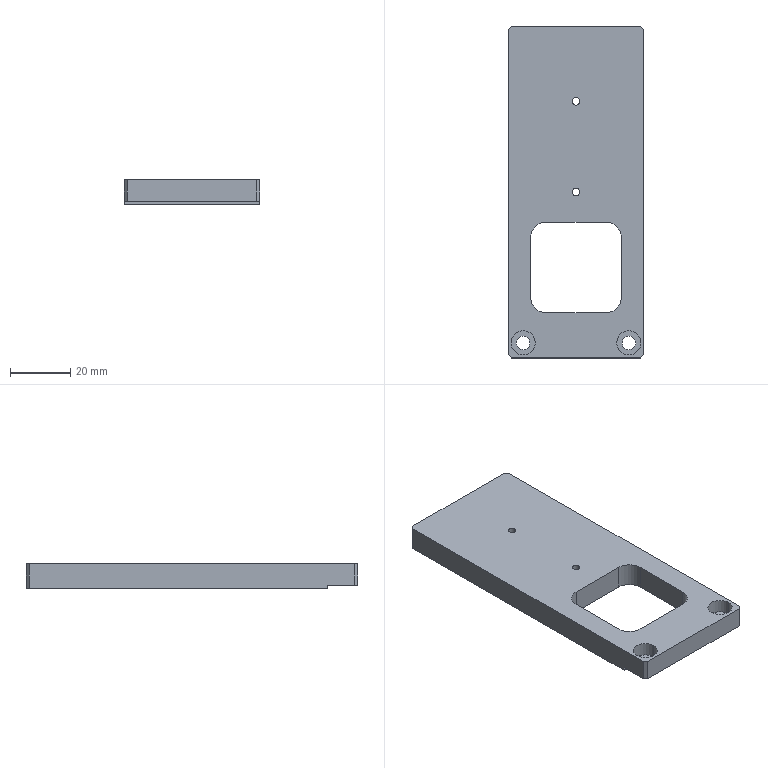Part | SolidWorks | features HoleWzd 2, ICE 2, Chamfer 1, Extrusion 1 | 1 solid | 34 faces | box 45 x 110 x 8 mm | volume 31489 mm3 | plane 18 | cylinder 16 | commonest cylinder face diameters 2.5 x4 4.5 x4 8 x4 10 x4
STEP:
#1=CARTESIAN_POINT('',(-1.25,30.,-4.));
#2=VERTEX_POINT('',#1);
#3=CARTESIAN_POINT('',(1.25,30.,-4.));
#4=VERTEX_POINT('',#3);
#5=CARTESIAN_POINT('',(0.,30.,-4.));
#6=DIRECTION('',(0.,0.,1.));
#7=DIRECTION('',(1.,0.,0.));
#8=AXIS2_PLACEMENT_3D('',#5,#6,#7);
#9=CIRCLE('',#8,1.25);
#10=EDGE_CURVE('',#2,#4,#9,.T.);
#11=ORIENTED_EDGE('',*,*,#10,.F.);
#12=CARTESIAN_POINT('',(-1.25,30.,4.));
#13=VERTEX_POINT('',#12);
#14=CARTESIAN_POINT('',(-1.25,30.,4.));
#15=DIRECTION('',(0.,0.,1.));
#16=VECTOR('',#15,1000.);
#17=LINE('',#14,#16);
#18=EDGE_CURVE('',#2,#13,#17,.T.);
#19=ORIENTED_EDGE('',*,*,#18,.T.);
#20=CARTESIAN_POINT('',(1.25,30.,4.));
#21=VERTEX_POINT('',#20);
#22=CARTESIAN_POINT('',(0.,30.,4.));
#23=DIRECTION('',(0.,0.,1.));
#24=DIRECTION('',(1.,0.,0.));
#25=AXIS2_PLACEMENT_3D('',#22,#23,#24);
#26=CIRCLE('',#25,1.25);
#27=EDGE_CURVE('',#13,#21,#26,.T.);
#28=ORIENTED_EDGE('',*,*,#27,.T.);
#29=CARTESIAN_POINT('',(1.25,30.,4.));
#30=DIRECTION('',(0.,0.,1.));
#31=VECTOR('',#30,1000.);
#32=LINE('',#29,#31);
#33=EDGE_CURVE('',#4,#21,#32,.T.);
#34=ORIENTED_EDGE('',*,*,#33,.F.);
#35=EDGE_LOOP('',(#11,#19,#28,#34));
#36=FACE_OUTER_BOUND('',#35,.T.);
#37=CARTESIAN_POINT('',(0.,30.,4.));
#38=DIRECTION('',(0.,0.,1.));
#39=DIRECTION('',(1.,0.,0.));
#40=AXIS2_PLACEMENT_3D('',#37,#38,#39);
#41=CYLINDRICAL_SURFACE('',#40,1.25);
#42=ADVANCED_FACE('',(#36),#41,.F.);
#43=CARTESIAN_POINT('',(-1.25,0.,-4.));
#44=VERTEX_POINT('',#43);
#45=CARTESIAN_POINT('',(1.25,0.,-4.));
#46=VERTEX_POINT('',#45);
#47=CARTESIAN_POINT('',(0.,0.,-4.));
#48=DIRECTION('',(0.,0.,1.));
#49=DIRECTION('',(1.,0.,0.));
#50=AXIS2_PLACEMENT_3D('',#47,#48,#49);
#51=CIRCLE('',#50,1.25);
#52=EDGE_CURVE('',#44,#46,#51,.T.);
#53=ORIENTED_EDGE('',*,*,#52,.F.);
#54=CARTESIAN_POINT('',(-1.25,0.,4.));
#55=VERTEX_POINT('',#54);
#56=CARTESIAN_POINT('',(-1.25,0.,4.));
#57=DIRECTION('',(0.,0.,1.));
#58=VECTOR('',#57,1000.);
#59=LINE('',#56,#58);
#60=EDGE_CURVE('',#44,#55,#59,.T.);
#61=ORIENTED_EDGE('',*,*,#60,.T.);
#62=CARTESIAN_POINT('',(1.25,0.,4.));
#63=VERTEX_POINT('',#62);
#64=CARTESIAN_POINT('',(0.,0.,4.));
#65=DIRECTION('',(0.,0.,1.));
#66=DIRECTION('',(1.,0.,0.));
#67=AXIS2_PLACEMENT_3D('',#64,#65,#66);
#68=CIRCLE('',#67,1.25);
#69=EDGE_CURVE('',#55,#63,#68,.T.);
#70=ORIENTED_EDGE('',*,*,#69,.T.);
#71=CARTESIAN_POINT('',(1.25,0.,4.));
#72=DIRECTION('',(0.,0.,1.));
#73=VECTOR('',#72,1000.);
#74=LINE('',#71,#73);
#75=EDGE_CURVE('',#46,#63,#74,.T.);
#76=ORIENTED_EDGE('',*,*,#75,.F.);
#77=EDGE_LOOP('',(#53,#61,#70,#76));
#78=FACE_OUTER_BOUND('',#77,.T.);
#79=CARTESIAN_POINT('',(0.,0.,4.));
#80=DIRECTION('',(0.,0.,1.));
#81=DIRECTION('',(1.,0.,0.));
#82=AXIS2_PLACEMENT_3D('',#79,#80,#81);
#83=CYLINDRICAL_SURFACE('',#82,1.25);
#84=ADVANCED_FACE('',(#78),#83,.F.);
#85=CARTESIAN_POINT('',(-21.5,-50.,-0.6));
#86=VERTEX_POINT('',#85);
#87=CARTESIAN_POINT('',(-13.5,-50.,-0.6));
#88=VERTEX_POINT('',#87);
#89=CARTESIAN_POINT('',(-17.5,-50.,-0.6));
#90=DIRECTION('',(0.,0.,1.));
#91=DIRECTION('',(1.,0.,0.));
#92=AXIS2_PLACEMENT_3D('',#89,#90,#91);
#93=CIRCLE('',#92,4.);
#94=EDGE_CURVE('',#86,#88,#93,.T.);
#95=ORIENTED_EDGE('',*,*,#94,.F.);
#96=CARTESIAN_POINT('',(-21.5,-50.,4.));
#97=VERTEX_POINT('',#96);
#98=CARTESIAN_POINT('',(-21.5,-50.,4.));
#99=DIRECTION('',(0.,0.,1.));
#100=VECTOR('',#99,1000.);
#101=LINE('',#98,#100);
#102=EDGE_CURVE('',#86,#97,#101,.T.);
#103=ORIENTED_EDGE('',*,*,#102,.T.);
#104=CARTESIAN_POINT('',(-13.5,-50.,4.));
#105=VERTEX_POINT('',#104);
#106=CARTESIAN_POINT('',(-17.5,-50.,4.));
#107=DIRECTION('',(0.,0.,1.));
#108=DIRECTION('',(1.,0.,0.));
#109=AXIS2_PLACEMENT_3D('',#106,#107,#108);
#110=CIRCLE('',#109,4.);
#111=EDGE_CURVE('',#97,#105,#110,.T.);
#112=ORIENTED_EDGE('',*,*,#111,.T.);
#113=CARTESIAN_POINT('',(-13.5,-50.,4.));
#114=DIRECTION('',(0.,0.,1.));
#115=VECTOR('',#114,1000.);
#116=LINE('',#113,#115);
#117=EDGE_CURVE('',#88,#105,#116,.T.);
#118=ORIENTED_EDGE('',*,*,#117,.F.);
#119=EDGE_LOOP('',(#95,#103,#112,#118));
#120=FACE_OUTER_BOUND('',#119,.T.);
#121=CARTESIAN_POINT('',(-17.5,-50.,4.));
#122=DIRECTION('',(0.,0.,1.));
#123=DIRECTION('',(1.,0.,0.));
#124=AXIS2_PLACEMENT_3D('',#121,#122,#123);
#125=CYLINDRICAL_SURFACE('',#124,4.);
#126=ADVANCED_FACE('',(#120),#125,.F.);
#127=CARTESIAN_POINT('',(-15.25,-50.,-3.));
#128=VERTEX_POINT('',#127);
#129=CARTESIAN_POINT('',(-19.75,-50.,-3.));
#130=VERTEX_POINT('',#129);
#131=CARTESIAN_POINT('',(-17.5,-50.,-3.));
#132=DIRECTION('',(0.,0.,-1.));
#133=DIRECTION('',(1.,0.,0.));
#134=AXIS2_PLACEMENT_3D('',#131,#132,#133);
#135=CIRCLE('',#134,2.25);
#136=EDGE_CURVE('',#128,#130,#135,.T.);
#137=ORIENTED_EDGE('',*,*,#136,.T.);
#138=CARTESIAN_POINT('',(-19.75,-50.,-0.6));
#139=VERTEX_POINT('',#138);
#140=CARTESIAN_POINT('',(-19.75,-50.,4.));
#141=DIRECTION('',(0.,0.,1.));
#142=VECTOR('',#141,1000.);
#143=LINE('',#140,#142);
#144=EDGE_CURVE('',#130,#139,#143,.T.);
#145=ORIENTED_EDGE('',*,*,#144,.T.);
#146=CARTESIAN_POINT('',(-15.25,-50.,-0.6));
#147=VERTEX_POINT('',#146);
#148=CARTESIAN_POINT('',(-17.5,-50.,-0.6));
#149=DIRECTION('',(0.,0.,1.));
#150=DIRECTION('',(1.,0.,0.));
#151=AXIS2_PLACEMENT_3D('',#148,#149,#150);
#152=CIRCLE('',#151,2.25);
#153=EDGE_CURVE('',#139,#147,#152,.T.);
#154=ORIENTED_EDGE('',*,*,#153,.T.);
#155=CARTESIAN_POINT('',(-15.25,-50.,4.));
#156=DIRECTION('',(0.,0.,1.));
#157=VECTOR('',#156,1000.);
#158=LINE('',#155,#157);
#159=EDGE_CURVE('',#128,#147,#158,.T.);
#160=ORIENTED_EDGE('',*,*,#159,.F.);
#161=EDGE_LOOP('',(#137,#145,#154,#160));
#162=FACE_OUTER_BOUND('',#161,.T.);
#163=CARTESIAN_POINT('',(-17.5,-50.,4.));
#164=DIRECTION('',(0.,0.,1.));
#165=DIRECTION('',(1.,0.,0.));
#166=AXIS2_PLACEMENT_3D('',#163,#164,#165);
#167=CYLINDRICAL_SURFACE('',#166,2.25);
#168=ADVANCED_FACE('',(#162),#167,.F.);
#169=CARTESIAN_POINT('',(13.5,-50.,-0.6));
#170=VERTEX_POINT('',#169);
#171=CARTESIAN_POINT('',(21.5,-50.,-0.6));
#172=VERTEX_POINT('',#171);
#173=CARTESIAN_POINT('',(17.5,-50.,-0.6));
#174=DIRECTION('',(0.,0.,1.));
#175=DIRECTION('',(1.,0.,0.));
#176=AXIS2_PLACEMENT_3D('',#173,#174,#175);
#177=CIRCLE('',#176,4.);
#178=EDGE_CURVE('',#170,#172,#177,.T.);
#179=ORIENTED_EDGE('',*,*,#178,.F.);
#180=CARTESIAN_POINT('',(13.5,-50.,4.));
#181=VERTEX_POINT('',#180);
#182=CARTESIAN_POINT('',(13.5,-50.,4.));
#183=DIRECTION('',(0.,0.,1.));
#184=VECTOR('',#183,1000.);
#185=LINE('',#182,#184);
#186=EDGE_CURVE('',#170,#181,#185,.T.);
#187=ORIENTED_EDGE('',*,*,#186,.T.);
#188=CARTESIAN_POINT('',(21.5,-50.,4.));
#189=VERTEX_POINT('',#188);
#190=CARTESIAN_POINT('',(17.5,-50.,4.));
#191=DIRECTION('',(0.,0.,1.));
#192=DIRECTION('',(1.,0.,0.));
#193=AXIS2_PLACEMENT_3D('',#190,#191,#192);
#194=CIRCLE('',#193,4.);
#195=EDGE_CURVE('',#181,#189,#194,.T.);
#196=ORIENTED_EDGE('',*,*,#195,.T.);
#197=CARTESIAN_POINT('',(21.5,-50.,4.));
#198=DIRECTION('',(0.,0.,1.));
#199=VECTOR('',#198,1000.);
#200=LINE('',#197,#199);
#201=EDGE_CURVE('',#172,#189,#200,.T.);
#202=ORIENTED_EDGE('',*,*,#201,.F.);
#203=EDGE_LOOP('',(#179,#187,#196,#202));
#204=FACE_OUTER_BOUND('',#203,.T.);
#205=CARTESIAN_POINT('',(17.5,-50.,4.));
#206=DIRECTION('',(0.,0.,1.));
#207=DIRECTION('',(1.,0.,0.));
#208=AXIS2_PLACEMENT_3D('',#205,#206,#207);
#209=CYLINDRICAL_SURFACE('',#208,4.);
#210=ADVANCED_FACE('',(#204),#209,.F.);
#211=CARTESIAN_POINT('',(19.75,-50.,-3.));
#212=VERTEX_POINT('',#211);
#213=CARTESIAN_POINT('',(15.25,-50.,-3.));
#214=VERTEX_POINT('',#213);
#215=CARTESIAN_POINT('',(17.5,-50.,-3.));
#216=DIRECTION('',(0.,0.,-1.));
#217=DIRECTION('',(1.,0.,0.));
#218=AXIS2_PLACEMENT_3D('',#215,#216,#217);
#219=CIRCLE('',#218,2.25);
#220=EDGE_CURVE('',#212,#214,#219,.T.);
#221=ORIENTED_EDGE('',*,*,#220,.T.);
#222=CARTESIAN_POINT('',(15.25,-50.,-0.6));
#223=VERTEX_POINT('',#222);
#224=CARTESIAN_POINT('',(15.25,-50.,4.));
#225=DIRECTION('',(0.,0.,1.));
#226=VECTOR('',#225,1000.);
#227=LINE('',#224,#226);
#228=EDGE_CURVE('',#214,#223,#227,.T.);
#229=ORIENTED_EDGE('',*,*,#228,.T.);
#230=CARTESIAN_POINT('',(19.75,-50.,-0.6));
#231=VERTEX_POINT('',#230);
#232=CARTESIAN_POINT('',(17.5,-50.,-0.6));
#233=DIRECTION('',(0.,0.,1.));
#234=DIRECTION('',(1.,0.,0.));
#235=AXIS2_PLACEMENT_3D('',#232,#233,#234);
#236=CIRCLE('',#235,2.25);
#237=EDGE_CURVE('',#223,#231,#236,.T.);
#238=ORIENTED_EDGE('',*,*,#237,.T.);
#239=CARTESIAN_POINT('',(19.75,-50.,4.));
#240=DIRECTION('',(0.,0.,1.));
#241=VECTOR('',#240,1000.);
#242=LINE('',#239,#241);
#243=EDGE_CURVE('',#212,#231,#242,.T.);
#244=ORIENTED_EDGE('',*,*,#243,.F.);
#245=EDGE_LOOP('',(#221,#229,#238,#244));
#246=FACE_OUTER_BOUND('',#245,.T.);
#247=CARTESIAN_POINT('',(17.5,-50.,4.));
#248=DIRECTION('',(0.,0.,1.));
#249=DIRECTION('',(1.,0.,0.));
#250=AXIS2_PLACEMENT_3D('',#247,#248,#249);
#251=CYLINDRICAL_SURFACE('',#250,2.25);
#252=ADVANCED_FACE('',(#246),#251,.F.);
#253=CARTESIAN_POINT('',(10.,-10.,4.));
#254=VERTEX_POINT('',#253);
#255=CARTESIAN_POINT('',(-10.,-10.,4.));
#256=VERTEX_POINT('',#255);
#257=CARTESIAN_POINT('',(10.,-10.,4.));
#258=DIRECTION('',(-1.,0.,0.));
#259=VECTOR('',#258,1000.);
#260=LINE('',#257,#259);
#261=EDGE_CURVE('',#254,#256,#260,.T.);
#262=ORIENTED_EDGE('',*,*,#261,.F.);
#263=CARTESIAN_POINT('',(15.,-15.,4.));
#264=VERTEX_POINT('',#263);
#265=CARTESIAN_POINT('',(10.,-15.,4.));
#266=DIRECTION('',(0.,0.,1.));
#267=DIRECTION('',(-1.,0.,0.));
#268=AXIS2_PLACEMENT_3D('',#265,#266,#267);
#269=CIRCLE('',#268,5.);
#270=EDGE_CURVE('',#264,#254,#269,.T.);
#271=ORIENTED_EDGE('',*,*,#270,.F.);
#272=CARTESIAN_POINT('',(15.,-35.,4.));
#273=VERTEX_POINT('',#272);
#274=CARTESIAN_POINT('',(15.,-15.,4.));
#275=DIRECTION('',(0.,1.,0.));
#276=VECTOR('',#275,1000.);
#277=LINE('',#274,#276);
#278=EDGE_CURVE('',#273,#264,#277,.T.);
#279=ORIENTED_EDGE('',*,*,#278,.F.);
#280=CARTESIAN_POINT('',(10.,-40.,4.));
#281=VERTEX_POINT('',#280);
#282=CARTESIAN_POINT('',(10.,-35.,4.));
#283=DIRECTION('',(0.,0.,1.));
#284=DIRECTION('',(-1.,0.,0.));
#285=AXIS2_PLACEMENT_3D('',#282,#283,#284);
#286=CIRCLE('',#285,5.);
#287=EDGE_CURVE('',#281,#273,#286,.T.);
#288=ORIENTED_EDGE('',*,*,#287,.F.);
#289=CARTESIAN_POINT('',(-10.,-40.,4.));
#290=VERTEX_POINT('',#289);
#291=CARTESIAN_POINT('',(10.,-40.,4.));
#292=DIRECTION('',(1.,0.,0.));
#293=VECTOR('',#292,1000.);
#294=LINE('',#291,#293);
#295=EDGE_CURVE('',#290,#281,#294,.T.);
#296=ORIENTED_EDGE('',*,*,#295,.F.);
#297=CARTESIAN_POINT('',(-15.,-35.,4.));
#298=VERTEX_POINT('',#297);
#299=CARTESIAN_POINT('',(-10.,-35.,4.));
#300=DIRECTION('',(0.,0.,1.));
#301=DIRECTION('',(-1.,0.,0.));
#302=AXIS2_PLACEMENT_3D('',#299,#300,#301);
#303=CIRCLE('',#302,5.);
#304=EDGE_CURVE('',#298,#290,#303,.T.);
#305=ORIENTED_EDGE('',*,*,#304,.F.);
#306=CARTESIAN_POINT('',(-15.,-15.,4.));
#307=VERTEX_POINT('',#306);
#308=CARTESIAN_POINT('',(-15.,-15.,4.));
#309=DIRECTION('',(0.,-1.,0.));
#310=VECTOR('',#309,1000.);
#311=LINE('',#308,#310);
#312=EDGE_CURVE('',#307,#298,#311,.T.);
#313=ORIENTED_EDGE('',*,*,#312,.F.);
#314=CARTESIAN_POINT('',(-10.,-15.,4.));
#315=DIRECTION('',(0.,0.,1.));
#316=DIRECTION('',(1.,0.,0.));
#317=AXIS2_PLACEMENT_3D('',#314,#315,#316);
#318=CIRCLE('',#317,5.);
#319=EDGE_CURVE('',#256,#307,#318,.T.);
#320=ORIENTED_EDGE('',*,*,#319,.F.);
#321=EDGE_LOOP('',(#262,#271,#279,#288,#296,#305,#313,#320));
#322=FACE_BOUND('',#321,.T.);
#323=CARTESIAN_POINT('',(0.,30.,4.));
#324=DIRECTION('',(0.,0.,1.));
#325=DIRECTION('',(1.,0.,0.));
#326=AXIS2_PLACEMENT_3D('',#323,#324,#325);
#327=CIRCLE('',#326,1.25);
#328=EDGE_CURVE('',#21,#13,#327,.T.);
#329=ORIENTED_EDGE('',*,*,#328,.F.);
#330=ORIENTED_EDGE('',*,*,#27,.F.);
#331=EDGE_LOOP('',(#329,#330));
#332=FACE_BOUND('',#331,.T.);
#333=CARTESIAN_POINT('',(21.5,55.,4.));
#334=VERTEX_POINT('',#333);
#335=CARTESIAN_POINT('',(-21.5,55.,4.));
#336=VERTEX_POINT('',#335);
#337=CARTESIAN_POINT('',(-22.5,55.,4.));
#338=DIRECTION('',(-1.,0.,0.));
#339=VECTOR('',#338,1000.);
#340=LINE('',#337,#339);
#341=EDGE_CURVE('',#334,#336,#340,.T.);
#342=ORIENTED_EDGE('',*,*,#341,.T.);
#343=CARTESIAN_POINT('',(-22.5,54.,4.));
#344=VERTEX_POINT('',#343);
#345=CARTESIAN_POINT('',(-22.5,54.,4.));
#346=DIRECTION('',(-0.7071,-0.7071,0.));
#347=VECTOR('',#346,1000.);
#348=LINE('',#345,#347);
#349=EDGE_CURVE('',#336,#344,#348,.T.);
#350=ORIENTED_EDGE('',*,*,#349,.T.);
#351=CARTESIAN_POINT('',(-22.5,-54.,4.));
#352=VERTEX_POINT('',#351);
#353=CARTESIAN_POINT('',(-22.5,-55.,4.));
#354=DIRECTION('',(0.,-1.,0.));
#355=VECTOR('',#354,1000.);
#356=LINE('',#353,#355);
#357=EDGE_CURVE('',#344,#352,#356,.T.);
#358=ORIENTED_EDGE('',*,*,#357,.T.);
#359=CARTESIAN_POINT('',(-21.5,-55.,4.));
#360=VERTEX_POINT('',#359);
#361=CARTESIAN_POINT('',(-21.5,-55.,4.));
#362=DIRECTION('',(0.7071,-0.7071,0.));
#363=VECTOR('',#362,1000.);
#364=LINE('',#361,#363);
#365=EDGE_CURVE('',#352,#360,#364,.T.);
#366=ORIENTED_EDGE('',*,*,#365,.T.);
#367=CARTESIAN_POINT('',(21.5,-55.,4.));
#368=VERTEX_POINT('',#367);
#369=CARTESIAN_POINT('',(-22.5,-55.,4.));
#370=DIRECTION('',(1.,0.,0.));
#371=VECTOR('',#370,1000.);
#372=LINE('',#369,#371);
#373=EDGE_CURVE('',#360,#368,#372,.T.);
#374=ORIENTED_EDGE('',*,*,#373,.T.);
#375=CARTESIAN_POINT('',(22.5,-54.,4.));
#376=VERTEX_POINT('',#375);
#377=CARTESIAN_POINT('',(22.5,-54.,4.));
#378=DIRECTION('',(0.7071,0.7071,0.));
#379=VECTOR('',#378,1000.);
#380=LINE('',#377,#379);
#381=EDGE_CURVE('',#368,#376,#380,.T.);
#382=ORIENTED_EDGE('',*,*,#381,.T.);
#383=CARTESIAN_POINT('',(22.5,54.,4.));
#384=VERTEX_POINT('',#383);
#385=CARTESIAN_POINT('',(22.5,-55.,4.));
#386=DIRECTION('',(0.,1.,0.));
#387=VECTOR('',#386,1000.);
#388=LINE('',#385,#387);
#389=EDGE_CURVE('',#376,#384,#388,.T.);
#390=ORIENTED_EDGE('',*,*,#389,.T.);
#391=CARTESIAN_POINT('',(21.5,55.,4.));
#392=DIRECTION('',(-0.7071,0.7071,0.));
#393=VECTOR('',#392,1000.);
#394=LINE('',#391,#393);
#395=EDGE_CURVE('',#384,#334,#394,.T.);
#396=ORIENTED_EDGE('',*,*,#395,.T.);
#397=EDGE_LOOP('',(#342,#350,#358,#366,#374,#382,#390,#396));
#398=FACE_OUTER_BOUND('',#397,.T.);
#399=CARTESIAN_POINT('',(17.5,-50.,4.));
#400=DIRECTION('',(0.,0.,1.));
#401=DIRECTION('',(1.,0.,0.));
#402=AXIS2_PLACEMENT_3D('',#399,#400,#401);
#403=CIRCLE('',#402,4.);
#404=EDGE_CURVE('',#189,#181,#403,.T.);
#405=ORIENTED_EDGE('',*,*,#404,.F.);
#406=ORIENTED_EDGE('',*,*,#195,.F.);
#407=EDGE_LOOP('',(#405,#406));
#408=FACE_BOUND('',#407,.T.);
#409=CARTESIAN_POINT('',(-17.5,-50.,4.));
#410=DIRECTION('',(0.,0.,1.));
#411=DIRECTION('',(1.,0.,0.));
#412=AXIS2_PLACEMENT_3D('',#409,#410,#411);
#413=CIRCLE('',#412,4.);
#414=EDGE_CURVE('',#105,#97,#413,.T.);
#415=ORIENTED_EDGE('',*,*,#414,.F.);
#416=ORIENTED_EDGE('',*,*,#111,.F.);
#417=EDGE_LOOP('',(#415,#416));
#418=FACE_BOUND('',#417,.T.);
#419=CARTESIAN_POINT('',(0.,0.,4.));
#420=DIRECTION('',(0.,0.,1.));
#421=DIRECTION('',(1.,0.,0.));
#422=AXIS2_PLACEMENT_3D('',#419,#420,#421);
#423=CIRCLE('',#422,1.25);
#424=EDGE_CURVE('',#63,#55,#423,.T.);
#425=ORIENTED_EDGE('',*,*,#424,.F.);
#426=ORIENTED_EDGE('',*,*,#69,.F.);
#427=EDGE_LOOP('',(#425,#426));
#428=FACE_BOUND('',#427,.T.);
#429=CARTESIAN_POINT('',(0.,0.,4.));
#430=DIRECTION('',(0.,0.,-1.));
#431=DIRECTION('',(-1.,0.,0.));
#432=AXIS2_PLACEMENT_3D('',#429,#430,#431);
#433=PLANE('',#432);
#434=ADVANCED_FACE('',(#322,#332,#398,#408,#418,#428),#433,.F.);
#435=CARTESIAN_POINT('',(22.5,-45.,-4.));
#436=VERTEX_POINT('',#435);
#437=CARTESIAN_POINT('',(22.5,54.,-4.));
#438=VERTEX_POINT('',#437);
#439=CARTESIAN_POINT('',(22.5,-55.,-4.));
#440=DIRECTION('',(0.,1.,0.));
#441=VECTOR('',#440,1000.);
#442=LINE('',#439,#441);
#443=EDGE_CURVE('',#436,#438,#442,.T.);
#444=ORIENTED_EDGE('',*,*,#443,.T.);
#445=CARTESIAN_POINT('',(22.5,54.,4.));
#446=DIRECTION('',(0.,0.,1.));
#447=VECTOR('',#446,1000.);
#448=LINE('',#445,#447);
#449=EDGE_CURVE('',#438,#384,#448,.T.);
#450=ORIENTED_EDGE('',*,*,#449,.T.);
#451=ORIENTED_EDGE('',*,*,#389,.F.);
#452=CARTESIAN_POINT('',(22.5,-54.,-3.));
#453=VERTEX_POINT('',#452);
#454=CARTESIAN_POINT('',(22.5,-54.,4.));
#455=DIRECTION('',(0.,0.,-1.));
#456=VECTOR('',#455,1000.);
#457=LINE('',#454,#456);
#458=EDGE_CURVE('',#376,#453,#457,.T.);
#459=ORIENTED_EDGE('',*,*,#458,.T.);
#460=CARTESIAN_POINT('',(22.5,-45.,-3.));
#461=VERTEX_POINT('',#460);
#462=CARTESIAN_POINT('',(22.5,-55.,-3.));
#463=DIRECTION('',(0.,-1.,0.));
#464=VECTOR('',#463,1000.);
#465=LINE('',#462,#464);
#466=EDGE_CURVE('',#461,#453,#465,.T.);
#467=ORIENTED_EDGE('',*,*,#466,.F.);
#468=CARTESIAN_POINT('',(22.5,-45.,-4.));
#469=DIRECTION('',(0.,0.,1.));
#470=VECTOR('',#469,1000.);
#471=LINE('',#468,#470);
#472=EDGE_CURVE('',#436,#461,#471,.T.);
#473=ORIENTED_EDGE('',*,*,#472,.F.);
#474=EDGE_LOOP('',(#444,#450,#451,#459,#467,#473));
#475=FACE_OUTER_BOUND('',#474,.T.);
#476=CARTESIAN_POINT('',(22.5,-55.,4.));
#477=DIRECTION('',(-1.,0.,0.));
#478=DIRECTION('',(0.,0.,1.));
#479=AXIS2_PLACEMENT_3D('',#476,#477,#478);
#480=PLANE('',#479);
#481=ADVANCED_FACE('',(#475),#480,.F.);
#482=CARTESIAN_POINT('',(21.5,55.,-4.));
#483=VERTEX_POINT('',#482);
#484=CARTESIAN_POINT('',(-21.5,55.,-4.));
#485=VERTEX_POINT('',#484);
#486=CARTESIAN_POINT('',(-22.5,55.,-4.));
#487=DIRECTION('',(-1.,0.,0.));
#488=VECTOR('',#487,1000.);
#489=LINE('',#486,#488);
#490=EDGE_CURVE('',#483,#485,#489,.T.);
#491=ORIENTED_EDGE('',*,*,#490,.T.);
#492=CARTESIAN_POINT('',(-21.5,55.,4.));
#493=DIRECTION('',(0.,0.,1.));
#494=VECTOR('',#493,1000.);
#495=LINE('',#492,#494);
#496=EDGE_CURVE('',#485,#336,#495,.T.);
#497=ORIENTED_EDGE('',*,*,#496,.T.);
#498=ORIENTED_EDGE('',*,*,#341,.F.);
#499=CARTESIAN_POINT('',(21.5,55.,4.));
#500=DIRECTION('',(0.,0.,-1.));
#501=VECTOR('',#500,1000.);
#502=LINE('',#499,#501);
#503=EDGE_CURVE('',#334,#483,#502,.T.);
#504=ORIENTED_EDGE('',*,*,#503,.T.);
#505=EDGE_LOOP('',(#491,#497,#498,#504));
#506=FACE_OUTER_BOUND('',#505,.T.);
#507=CARTESIAN_POINT('',(-22.5,55.,4.));
#508=DIRECTION('',(0.,-1.,0.));
#509=DIRECTION('',(0.,0.,-1.));
#510=AXIS2_PLACEMENT_3D('',#507,#508,#509);
#511=PLANE('',#510);
#512=ADVANCED_FACE('',(#506),#511,.F.);
#513=ORIENTED_EDGE('',*,*,#357,.F.);
#514=CARTESIAN_POINT('',(-22.5,54.,-4.));
#515=VERTEX_POINT('',#514);
#516=CARTESIAN_POINT('',(-22.5,54.,4.));
#517=DIRECTION('',(0.,0.,-1.));
#518=VECTOR('',#517,1000.);
#519=LINE('',#516,#518);
#520=EDGE_CURVE('',#344,#515,#519,.T.);
#521=ORIENTED_EDGE('',*,*,#520,.T.);
#522=CARTESIAN_POINT('',(-22.5,-45.,-4.));
#523=VERTEX_POINT('',#522);
#524=CARTESIAN_POINT('',(-22.5,-55.,-4.));
#525=DIRECTION('',(0.,-1.,0.));
#526=VECTOR('',#525,1000.);
#527=LINE('',#524,#526);
#528=EDGE_CURVE('',#515,#523,#527,.T.);
#529=ORIENTED_EDGE('',*,*,#528,.T.);
#530=CARTESIAN_POINT('',(-22.5,-45.,-3.));
#531=VERTEX_POINT('',#530);
#532=CARTESIAN_POINT('',(-22.5,-45.,-4.));
#533=DIRECTION('',(0.,0.,1.));
#534=VECTOR('',#533,1000.);
#535=LINE('',#532,#534);
#536=EDGE_CURVE('',#523,#531,#535,.T.);
#537=ORIENTED_EDGE('',*,*,#536,.T.);
#538=CARTESIAN_POINT('',(-22.5,-54.,-3.));
#539=VERTEX_POINT('',#538);
#540=CARTESIAN_POINT('',(-22.5,-55.,-3.));
#541=DIRECTION('',(0.,-1.,0.));
#542=VECTOR('',#541,1000.);
#543=LINE('',#540,#542);
#544=EDGE_CURVE('',#531,#539,#543,.T.);
#545=ORIENTED_EDGE('',*,*,#544,.T.);
#546=CARTESIAN_POINT('',(-22.5,-54.,4.));
#547=DIRECTION('',(0.,0.,1.));
#548=VECTOR('',#547,1000.);
#549=LINE('',#546,#548);
#550=EDGE_CURVE('',#539,#352,#549,.T.);
#551=ORIENTED_EDGE('',*,*,#550,.T.);
#552=EDGE_LOOP('',(#513,#521,#529,#537,#545,#551));
#553=FACE_OUTER_BOUND('',#552,.T.);
#554=CARTESIAN_POINT('',(-22.5,-55.,4.));
#555=DIRECTION('',(1.,0.,0.));
#556=DIRECTION('',(0.,0.,-1.));
#557=AXIS2_PLACEMENT_3D('',#554,#555,#556);
#558=PLANE('',#557);
#559=ADVANCED_FACE('',(#553),#558,.F.);
#560=ORIENTED_EDGE('',*,*,#373,.F.);
#561=CARTESIAN_POINT('',(-21.5,-55.,-3.));
#562=VERTEX_POINT('',#561);
#563=CARTESIAN_POINT('',(-21.5,-55.,4.));
#564=DIRECTION('',(0.,0.,-1.));
#565=VECTOR('',#564,1000.);
#566=LINE('',#563,#565);
#567=EDGE_CURVE('',#360,#562,#566,.T.);
#568=ORIENTED_EDGE('',*,*,#567,.T.);
#569=CARTESIAN_POINT('',(21.5,-55.,-3.));
#570=VERTEX_POINT('',#569);
#571=CARTESIAN_POINT('',(-22.5,-55.,-3.));
#572=DIRECTION('',(1.,0.,0.));
#573=VECTOR('',#572,1000.);
#574=LINE('',#571,#573);
#575=EDGE_CURVE('',#562,#570,#574,.T.);
#576=ORIENTED_EDGE('',*,*,#575,.T.);
#577=CARTESIAN_POINT('',(21.5,-55.,4.));
#578=DIRECTION('',(0.,0.,1.));
#579=VECTOR('',#578,1000.);
#580=LINE('',#577,#579);
#581=EDGE_CURVE('',#570,#368,#580,.T.);
#582=ORIENTED_EDGE('',*,*,#581,.T.);
#583=EDGE_LOOP('',(#560,#568,#576,#582));
#584=FACE_OUTER_BOUND('',#583,.T.);
#585=CARTESIAN_POINT('',(-22.5,-55.,4.));
#586=DIRECTION('',(0.,1.,0.));
#587=DIRECTION('',(0.,0.,1.));
#588=AXIS2_PLACEMENT_3D('',#585,#586,#587);
#589=PLANE('',#588);
#590=ADVANCED_FACE('',(#584),#589,.F.);
#591=CARTESIAN_POINT('',(15.,-15.,-4.));
#592=VERTEX_POINT('',#591);
#593=CARTESIAN_POINT('',(10.,-10.,-4.));
#594=VERTEX_POINT('',#593);
#595=CARTESIAN_POINT('',(10.,-15.,-4.));
#596=DIRECTION('',(0.,0.,1.));
#597=DIRECTION('',(-1.,0.,0.));
#598=AXIS2_PLACEMENT_3D('',#595,#596,#597);
#599=CIRCLE('',#598,5.);
#600=EDGE_CURVE('',#592,#594,#599,.T.);
#601=ORIENTED_EDGE('',*,*,#600,.T.);
#602=CARTESIAN_POINT('',(-10.,-10.,-4.));
#603=VERTEX_POINT('',#602);
#604=CARTESIAN_POINT('',(10.,-10.,-4.));
#605=DIRECTION('',(-1.,0.,0.));
#606=VECTOR('',#605,1000.);
#607=LINE('',#604,#606);
#608=EDGE_CURVE('',#594,#603,#607,.T.);
#609=ORIENTED_EDGE('',*,*,#608,.T.);
#610=CARTESIAN_POINT('',(-15.,-15.,-4.));
#611=VERTEX_POINT('',#610);
#612=CARTESIAN_POINT('',(-10.,-15.,-4.));
#613=DIRECTION('',(0.,0.,1.));
#614=DIRECTION('',(1.,0.,0.));
#615=AXIS2_PLACEMENT_3D('',#612,#613,#614);
#616=CIRCLE('',#615,5.);
#617=EDGE_CURVE('',#603,#611,#616,.T.);
#618=ORIENTED_EDGE('',*,*,#617,.T.);
#619=CARTESIAN_POINT('',(-15.,-35.,-4.));
#620=VERTEX_POINT('',#619);
#621=CARTESIAN_POINT('',(-15.,-15.,-4.));
#622=DIRECTION('',(0.,-1.,0.));
#623=VECTOR('',#622,1000.);
#624=LINE('',#621,#623);
#625=EDGE_CURVE('',#611,#620,#624,.T.);
#626=ORIENTED_EDGE('',*,*,#625,.T.);
#627=CARTESIAN_POINT('',(-10.,-40.,-4.));
#628=VERTEX_POINT('',#627);
#629=CARTESIAN_POINT('',(-10.,-35.,-4.));
#630=DIRECTION('',(0.,0.,1.));
#631=DIRECTION('',(-1.,0.,0.));
#632=AXIS2_PLACEMENT_3D('',#629,#630,#631);
#633=CIRCLE('',#632,5.);
#634=EDGE_CURVE('',#620,#628,#633,.T.);
#635=ORIENTED_EDGE('',*,*,#634,.T.);
#636=CARTESIAN_POINT('',(10.,-40.,-4.));
#637=VERTEX_POINT('',#636);
#638=CARTESIAN_POINT('',(10.,-40.,-4.));
#639=DIRECTION('',(1.,0.,0.));
#640=VECTOR('',#639,1000.);
#641=LINE('',#638,#640);
#642=EDGE_CURVE('',#628,#637,#641,.T.);
#643=ORIENTED_EDGE('',*,*,#642,.T.);
#644=CARTESIAN_POINT('',(15.,-35.,-4.));
#645=VERTEX_POINT('',#644);
#646=CARTESIAN_POINT('',(10.,-35.,-4.));
#647=DIRECTION('',(0.,0.,1.));
#648=DIRECTION('',(-1.,0.,0.));
#649=AXIS2_PLACEMENT_3D('',#646,#647,#648);
#650=CIRCLE('',#649,5.);
#651=EDGE_CURVE('',#637,#645,#650,.T.);
#652=ORIENTED_EDGE('',*,*,#651,.T.);
#653=CARTESIAN_POINT('',(15.,-15.,-4.));
#654=DIRECTION('',(0.,1.,0.));
#655=VECTOR('',#654,1000.);
#656=LINE('',#653,#655);
#657=EDGE_CURVE('',#645,#592,#656,.T.);
#658=ORIENTED_EDGE('',*,*,#657,.T.);
#659=EDGE_LOOP('',(#601,#609,#618,#626,#635,#643,#652,#658));
#660=FACE_BOUND('',#659,.T.);
#661=CARTESIAN_POINT('',(0.,30.,-4.));
#662=DIRECTION('',(0.,0.,1.));
#663=DIRECTION('',(1.,0.,0.));
#664=AXIS2_PLACEMENT_3D('',#661,#662,#663);
#665=CIRCLE('',#664,1.25);
#666=EDGE_CURVE('',#4,#2,#665,.T.);
#667=ORIENTED_EDGE('',*,*,#666,.T.);
#668=ORIENTED_EDGE('',*,*,#10,.T.);
#669=EDGE_LOOP('',(#667,#668));
#670=FACE_BOUND('',#669,.T.);
#671=CARTESIAN_POINT('',(0.,0.,-4.));
#672=DIRECTION('',(0.,0.,1.));
#673=DIRECTION('',(1.,0.,0.));
#674=AXIS2_PLACEMENT_3D('',#671,#672,#673);
#675=CIRCLE('',#674,1.25);
#676=EDGE_CURVE('',#46,#44,#675,.T.);
#677=ORIENTED_EDGE('',*,*,#676,.T.);
#678=ORIENTED_EDGE('',*,*,#52,.T.);
#679=EDGE_LOOP('',(#677,#678));
#680=FACE_BOUND('',#679,.T.);
#681=ORIENTED_EDGE('',*,*,#528,.F.);
#682=CARTESIAN_POINT('',(-38.25,38.25,-4.));
#683=DIRECTION('',(0.7071,0.7071,0.));
#684=VECTOR('',#683,1000.);
#685=LINE('',#682,#684);
#686=EDGE_CURVE('',#515,#485,#685,.T.);
#687=ORIENTED_EDGE('',*,*,#686,.T.);
#688=ORIENTED_EDGE('',*,*,#490,.F.);
#689=CARTESIAN_POINT('',(38.25,38.25,-4.));
#690=DIRECTION('',(0.7071,-0.7071,0.));
#691=VECTOR('',#690,1000.);
#692=LINE('',#689,#691);
#693=EDGE_CURVE('',#483,#438,#692,.T.);
#694=ORIENTED_EDGE('',*,*,#693,.T.);
#695=ORIENTED_EDGE('',*,*,#443,.F.);
#696=CARTESIAN_POINT('',(-22.5,-45.,-4.));
#697=DIRECTION('',(1.,0.,0.));
#698=VECTOR('',#697,1000.);
#699=LINE('',#696,#698);
#700=EDGE_CURVE('',#523,#436,#699,.T.);
#701=ORIENTED_EDGE('',*,*,#700,.F.);
#702=EDGE_LOOP('',(#681,#687,#688,#694,#695,#701));
#703=FACE_OUTER_BOUND('',#702,.T.);
#704=CARTESIAN_POINT('',(0.,0.,-4.));
#705=DIRECTION('',(0.,0.,-1.));
#706=DIRECTION('',(-1.,0.,0.));
#707=AXIS2_PLACEMENT_3D('',#704,#705,#706);
#708=PLANE('',#707);
#709=ADVANCED_FACE('',(#660,#670,#680,#703),#708,.T.);
#710=ORIENTED_EDGE('',*,*,#228,.F.);
#711=CARTESIAN_POINT('',(17.5,-50.,-3.));
#712=DIRECTION('',(0.,0.,-1.));
#713=DIRECTION('',(1.,0.,0.));
#714=AXIS2_PLACEMENT_3D('',#711,#712,#713);
#715=CIRCLE('',#714,2.25);
#716=EDGE_CURVE('',#214,#212,#715,.T.);
#717=ORIENTED_EDGE('',*,*,#716,.T.);
#718=ORIENTED_EDGE('',*,*,#243,.T.);
#719=CARTESIAN_POINT('',(17.5,-50.,-0.6));
#720=DIRECTION('',(0.,0.,1.));
#721=DIRECTION('',(1.,0.,0.));
#722=AXIS2_PLACEMENT_3D('',#719,#720,#721);
#723=CIRCLE('',#722,2.25);
#724=EDGE_CURVE('',#231,#223,#723,.T.);
#725=ORIENTED_EDGE('',*,*,#724,.T.);
#726=EDGE_LOOP('',(#710,#717,#718,#725));
#727=FACE_OUTER_BOUND('',#726,.T.);
#728=CARTESIAN_POINT('',(17.5,-50.,4.));
#729=DIRECTION('',(0.,0.,1.));
#730=DIRECTION('',(1.,0.,0.));
#731=AXIS2_PLACEMENT_3D('',#728,#729,#730);
#732=CYLINDRICAL_SURFACE('',#731,2.25);
#733=ADVANCED_FACE('',(#727),#732,.F.);
#734=ORIENTED_EDGE('',*,*,#724,.F.);
#735=ORIENTED_EDGE('',*,*,#237,.F.);
#736=EDGE_LOOP('',(#734,#735));
#737=FACE_BOUND('',#736,.T.);
#738=CARTESIAN_POINT('',(17.5,-50.,-0.6));
#739=DIRECTION('',(0.,0.,1.));
#740=DIRECTION('',(1.,0.,0.));
#741=AXIS2_PLACEMENT_3D('',#738,#739,#740);
#742=CIRCLE('',#741,4.);
#743=EDGE_CURVE('',#172,#170,#742,.T.);
#744=ORIENTED_EDGE('',*,*,#743,.T.);
#745=ORIENTED_EDGE('',*,*,#178,.T.);
#746=EDGE_LOOP('',(#744,#745));
#747=FACE_OUTER_BOUND('',#746,.T.);
#748=CARTESIAN_POINT('',(19.75,-50.,-0.6));
#749=DIRECTION('',(0.,0.,-1.));
#750=DIRECTION('',(-1.,0.,0.));
#751=AXIS2_PLACEMENT_3D('',#748,#749,#750);
#752=PLANE('',#751);
#753=ADVANCED_FACE('',(#737,#747),#752,.F.);
#754=ORIENTED_EDGE('',*,*,#186,.F.);
#755=ORIENTED_EDGE('',*,*,#743,.F.);
#756=ORIENTED_EDGE('',*,*,#201,.T.);
#757=ORIENTED_EDGE('',*,*,#404,.T.);
#758=EDGE_LOOP('',(#754,#755,#756,#757));
#759=FACE_OUTER_BOUND('',#758,.T.);
#760=CARTESIAN_POINT('',(17.5,-50.,4.));
#761=DIRECTION('',(0.,0.,1.));
#762=DIRECTION('',(1.,0.,0.));
#763=AXIS2_PLACEMENT_3D('',#760,#761,#762);
#764=CYLINDRICAL_SURFACE('',#763,4.);
#765=ADVANCED_FACE('',(#759),#764,.F.);
#766=ORIENTED_EDGE('',*,*,#144,.F.);
#767=CARTESIAN_POINT('',(-17.5,-50.,-3.));
#768=DIRECTION('',(0.,0.,-1.));
#769=DIRECTION('',(1.,0.,0.));
#770=AXIS2_PLACEMENT_3D('',#767,#768,#769);
#771=CIRCLE('',#770,2.25);
#772=EDGE_CURVE('',#130,#128,#771,.T.);
#773=ORIENTED_EDGE('',*,*,#772,.T.);
#774=ORIENTED_EDGE('',*,*,#159,.T.);
#775=CARTESIAN_POINT('',(-17.5,-50.,-0.6));
#776=DIRECTION('',(0.,0.,1.));
#777=DIRECTION('',(1.,0.,0.));
#778=AXIS2_PLACEMENT_3D('',#775,#776,#777);
#779=CIRCLE('',#778,2.25);
#780=EDGE_CURVE('',#147,#139,#779,.T.);
#781=ORIENTED_EDGE('',*,*,#780,.T.);
#782=EDGE_LOOP('',(#766,#773,#774,#781));
#783=FACE_OUTER_BOUND('',#782,.T.);
#784=CARTESIAN_POINT('',(-17.5,-50.,4.));
#785=DIRECTION('',(0.,0.,1.));
#786=DIRECTION('',(1.,0.,0.));
#787=AXIS2_PLACEMENT_3D('',#784,#785,#786);
#788=CYLINDRICAL_SURFACE('',#787,2.25);
#789=ADVANCED_FACE('',(#783),#788,.F.);
#790=ORIENTED_EDGE('',*,*,#780,.F.);
#791=ORIENTED_EDGE('',*,*,#153,.F.);
#792=EDGE_LOOP('',(#790,#791));
#793=FACE_BOUND('',#792,.T.);
#794=CARTESIAN_POINT('',(-17.5,-50.,-0.6));
#795=DIRECTION('',(0.,0.,1.));
#796=DIRECTION('',(1.,0.,0.));
#797=AXIS2_PLACEMENT_3D('',#794,#795,#796);
#798=CIRCLE('',#797,4.);
#799=EDGE_CURVE('',#88,#86,#798,.T.);
#800=ORIENTED_EDGE('',*,*,#799,.T.);
#801=ORIENTED_EDGE('',*,*,#94,.T.);
#802=EDGE_LOOP('',(#800,#801));
#803=FACE_OUTER_BOUND('',#802,.T.);
#804=CARTESIAN_POINT('',(-15.25,-50.,-0.6));
#805=DIRECTION('',(0.,0.,-1.));
#806=DIRECTION('',(-1.,0.,0.));
#807=AXIS2_PLACEMENT_3D('',#804,#805,#806);
#808=PLANE('',#807);
#809=ADVANCED_FACE('',(#793,#803),#808,.F.);
#810=ORIENTED_EDGE('',*,*,#102,.F.);
#811=ORIENTED_EDGE('',*,*,#799,.F.);
#812=ORIENTED_EDGE('',*,*,#117,.T.);
#813=ORIENTED_EDGE('',*,*,#414,.T.);
#814=EDGE_LOOP('',(#810,#811,#812,#813));
#815=FACE_OUTER_BOUND('',#814,.T.);
#816=CARTESIAN_POINT('',(-17.5,-50.,4.));
#817=DIRECTION('',(0.,0.,1.));
#818=DIRECTION('',(1.,0.,0.));
#819=AXIS2_PLACEMENT_3D('',#816,#817,#818);
#820=CYLINDRICAL_SURFACE('',#819,4.);
#821=ADVANCED_FACE('',(#815),#820,.F.);
#822=ORIENTED_EDGE('',*,*,#136,.F.);
#823=ORIENTED_EDGE('',*,*,#772,.F.);
#824=EDGE_LOOP('',(#822,#823));
#825=FACE_BOUND('',#824,.T.);
#826=ORIENTED_EDGE('',*,*,#575,.F.);
#827=CARTESIAN_POINT('',(-21.5,-55.,-3.));
#828=DIRECTION('',(-0.7071,0.7071,0.));
#829=VECTOR('',#828,1000.);
#830=LINE('',#827,#829);
#831=EDGE_CURVE('',#562,#539,#830,.T.);
#832=ORIENTED_EDGE('',*,*,#831,.T.);
#833=ORIENTED_EDGE('',*,*,#544,.F.);
#834=CARTESIAN_POINT('',(-22.5,-45.,-3.));
#835=DIRECTION('',(1.,0.,0.));
#836=VECTOR('',#835,1000.);
#837=LINE('',#834,#836);
#838=EDGE_CURVE('',#531,#461,#837,.T.);
#839=ORIENTED_EDGE('',*,*,#838,.T.);
#840=ORIENTED_EDGE('',*,*,#466,.T.);
#841=CARTESIAN_POINT('',(22.5,-54.,-3.));
#842=DIRECTION('',(-0.7071,-0.7071,0.));
#843=VECTOR('',#842,1000.);
#844=LINE('',#841,#843);
#845=EDGE_CURVE('',#453,#570,#844,.T.);
#846=ORIENTED_EDGE('',*,*,#845,.T.);
#847=EDGE_LOOP('',(#826,#832,#833,#839,#840,#846));
#848=FACE_OUTER_BOUND('',#847,.T.);
#849=ORIENTED_EDGE('',*,*,#220,.F.);
#850=ORIENTED_EDGE('',*,*,#716,.F.);
#851=EDGE_LOOP('',(#849,#850));
#852=FACE_BOUND('',#851,.T.);
#853=CARTESIAN_POINT('',(-22.5,-55.,-3.));
#854=DIRECTION('',(0.,0.,1.));
#855=DIRECTION('',(1.,0.,0.));
#856=AXIS2_PLACEMENT_3D('',#853,#854,#855);
#857=PLANE('',#856);
#858=ADVANCED_FACE('',(#825,#848,#852),#857,.F.);
#859=ORIENTED_EDGE('',*,*,#472,.T.);
#860=ORIENTED_EDGE('',*,*,#838,.F.);
#861=ORIENTED_EDGE('',*,*,#536,.F.);
#862=ORIENTED_EDGE('',*,*,#700,.T.);
#863=EDGE_LOOP('',(#859,#860,#861,#862));
#864=FACE_OUTER_BOUND('',#863,.T.);
#865=CARTESIAN_POINT('',(-22.5,-45.,-4.));
#866=DIRECTION('',(0.,1.,0.));
#867=DIRECTION('',(0.,0.,1.));
#868=AXIS2_PLACEMENT_3D('',#865,#866,#867);
#869=PLANE('',#868);
#870=ADVANCED_FACE('',(#864),#869,.F.);
#871=ORIENTED_EDGE('',*,*,#60,.F.);
#872=ORIENTED_EDGE('',*,*,#676,.F.);
#873=ORIENTED_EDGE('',*,*,#75,.T.);
#874=ORIENTED_EDGE('',*,*,#424,.T.);
#875=EDGE_LOOP('',(#871,#872,#873,#874));
#876=FACE_OUTER_BOUND('',#875,.T.);
#877=CARTESIAN_POINT('',(0.,0.,4.));
#878=DIRECTION('',(0.,0.,1.));
#879=DIRECTION('',(1.,0.,0.));
#880=AXIS2_PLACEMENT_3D('',#877,#878,#879);
#881=CYLINDRICAL_SURFACE('',#880,1.25);
#882=ADVANCED_FACE('',(#876),#881,.F.);
#883=ORIENTED_EDGE('',*,*,#18,.F.);
#884=ORIENTED_EDGE('',*,*,#666,.F.);
#885=ORIENTED_EDGE('',*,*,#33,.T.);
#886=ORIENTED_EDGE('',*,*,#328,.T.);
#887=EDGE_LOOP('',(#883,#884,#885,#886));
#888=FACE_OUTER_BOUND('',#887,.T.);
#889=CARTESIAN_POINT('',(0.,30.,4.));
#890=DIRECTION('',(0.,0.,1.));
#891=DIRECTION('',(1.,0.,0.));
#892=AXIS2_PLACEMENT_3D('',#889,#890,#891);
#893=CYLINDRICAL_SURFACE('',#892,1.25);
#894=ADVANCED_FACE('',(#888),#893,.F.);
#895=ORIENTED_EDGE('',*,*,#349,.F.);
#896=ORIENTED_EDGE('',*,*,#496,.F.);
#897=ORIENTED_EDGE('',*,*,#686,.F.);
#898=ORIENTED_EDGE('',*,*,#520,.F.);
#899=EDGE_LOOP('',(#895,#896,#897,#898));
#900=FACE_OUTER_BOUND('',#899,.T.);
#901=CARTESIAN_POINT('',(-22.5,54.,4.));
#902=DIRECTION('',(0.7071,-0.7071,0.));
#903=DIRECTION('',(0.,0.,-1.));
#904=AXIS2_PLACEMENT_3D('',#901,#902,#903);
#905=PLANE('',#904);
#906=ADVANCED_FACE('',(#900),#905,.F.);
#907=ORIENTED_EDGE('',*,*,#395,.F.);
#908=ORIENTED_EDGE('',*,*,#449,.F.);
#909=ORIENTED_EDGE('',*,*,#693,.F.);
#910=ORIENTED_EDGE('',*,*,#503,.F.);
#911=EDGE_LOOP('',(#907,#908,#909,#910));
#912=FACE_OUTER_BOUND('',#911,.T.);
#913=CARTESIAN_POINT('',(21.5,55.,4.));
#914=DIRECTION('',(-0.7071,-0.7071,0.));
#915=DIRECTION('',(0.,0.,-1.));
#916=AXIS2_PLACEMENT_3D('',#913,#914,#915);
#917=PLANE('',#916);
#918=ADVANCED_FACE('',(#912),#917,.F.);
#919=ORIENTED_EDGE('',*,*,#365,.F.);
#920=ORIENTED_EDGE('',*,*,#550,.F.);
#921=ORIENTED_EDGE('',*,*,#831,.F.);
#922=ORIENTED_EDGE('',*,*,#567,.F.);
#923=EDGE_LOOP('',(#919,#920,#921,#922));
#924=FACE_OUTER_BOUND('',#923,.T.);
#925=CARTESIAN_POINT('',(-21.5,-55.,4.));
#926=DIRECTION('',(0.7071,0.7071,0.));
#927=DIRECTION('',(0.,0.,-1.));
#928=AXIS2_PLACEMENT_3D('',#925,#926,#927);
#929=PLANE('',#928);
#930=ADVANCED_FACE('',(#924),#929,.F.);
#931=ORIENTED_EDGE('',*,*,#381,.F.);
#932=ORIENTED_EDGE('',*,*,#581,.F.);
#933=ORIENTED_EDGE('',*,*,#845,.F.);
#934=ORIENTED_EDGE('',*,*,#458,.F.);
#935=EDGE_LOOP('',(#931,#932,#933,#934));
#936=FACE_OUTER_BOUND('',#935,.T.);
#937=CARTESIAN_POINT('',(22.5,-54.,4.));
#938=DIRECTION('',(-0.7071,0.7071,0.));
#939=DIRECTION('',(0.,0.,-1.));
#940=AXIS2_PLACEMENT_3D('',#937,#938,#939);
#941=PLANE('',#940);
#942=ADVANCED_FACE('',(#936),#941,.F.);
#943=ORIENTED_EDGE('',*,*,#270,.T.);
#944=CARTESIAN_POINT('',(10.,-10.,-4.));
#945=DIRECTION('',(0.,0.,1.));
#946=VECTOR('',#945,1000.);
#947=LINE('',#944,#946);
#948=EDGE_CURVE('',#594,#254,#947,.T.);
#949=ORIENTED_EDGE('',*,*,#948,.F.);
#950=ORIENTED_EDGE('',*,*,#600,.F.);
#951=CARTESIAN_POINT('',(15.,-15.,-4.));
#952=DIRECTION('',(0.,0.,1.));
#953=VECTOR('',#952,1000.);
#954=LINE('',#951,#953);
#955=EDGE_CURVE('',#592,#264,#954,.T.);
#956=ORIENTED_EDGE('',*,*,#955,.T.);
#957=EDGE_LOOP('',(#943,#949,#950,#956));
#958=FACE_OUTER_BOUND('',#957,.T.);
#959=CARTESIAN_POINT('',(10.,-15.,-4.));
#960=DIRECTION('',(0.,0.,1.));
#961=DIRECTION('',(1.,0.,0.));
#962=AXIS2_PLACEMENT_3D('',#959,#960,#961);
#963=CYLINDRICAL_SURFACE('',#962,5.);
#964=ADVANCED_FACE('',(#958),#963,.F.);
#965=ORIENTED_EDGE('',*,*,#278,.T.);
#966=ORIENTED_EDGE('',*,*,#955,.F.);
#967=ORIENTED_EDGE('',*,*,#657,.F.);
#968=CARTESIAN_POINT('',(15.,-35.,-4.));
#969=DIRECTION('',(0.,0.,1.));
#970=VECTOR('',#969,1000.);
#971=LINE('',#968,#970);
#972=EDGE_CURVE('',#645,#273,#971,.T.);
#973=ORIENTED_EDGE('',*,*,#972,.T.);
#974=EDGE_LOOP('',(#965,#966,#967,#973));
#975=FACE_OUTER_BOUND('',#974,.T.);
#976=CARTESIAN_POINT('',(15.,-15.,-4.));
#977=DIRECTION('',(1.,0.,0.));
#978=DIRECTION('',(0.,1.,0.));
#979=AXIS2_PLACEMENT_3D('',#976,#977,#978);
#980=PLANE('',#979);
#981=ADVANCED_FACE('',(#975),#980,.F.);
#982=ORIENTED_EDGE('',*,*,#287,.T.);
#983=ORIENTED_EDGE('',*,*,#972,.F.);
#984=ORIENTED_EDGE('',*,*,#651,.F.);
#985=CARTESIAN_POINT('',(10.,-40.,-4.));
#986=DIRECTION('',(0.,0.,1.));
#987=VECTOR('',#986,1000.);
#988=LINE('',#985,#987);
#989=EDGE_CURVE('',#637,#281,#988,.T.);
#990=ORIENTED_EDGE('',*,*,#989,.T.);
#991=EDGE_LOOP('',(#982,#983,#984,#990));
#992=FACE_OUTER_BOUND('',#991,.T.);
#993=CARTESIAN_POINT('',(10.,-35.,-4.));
#994=DIRECTION('',(0.,0.,1.));
#995=DIRECTION('',(1.,0.,0.));
#996=AXIS2_PLACEMENT_3D('',#993,#994,#995);
#997=CYLINDRICAL_SURFACE('',#996,5.);
#998=ADVANCED_FACE('',(#992),#997,.F.);
#999=ORIENTED_EDGE('',*,*,#295,.T.);
#1000=ORIENTED_EDGE('',*,*,#989,.F.);
#1001=ORIENTED_EDGE('',*,*,#642,.F.);
#1002=CARTESIAN_POINT('',(-10.,-40.,-4.));
#1003=DIRECTION('',(0.,0.,1.));
#1004=VECTOR('',#1003,1000.);
#1005=LINE('',#1002,#1004);
#1006=EDGE_CURVE('',#628,#290,#1005,.T.);
#1007=ORIENTED_EDGE('',*,*,#1006,.T.);
#1008=EDGE_LOOP('',(#999,#1000,#1001,#1007));
#1009=FACE_OUTER_BOUND('',#1008,.T.);
#1010=CARTESIAN_POINT('',(10.,-40.,-4.));
#1011=DIRECTION('',(0.,-1.,0.));
#1012=DIRECTION('',(0.,0.,-1.));
#1013=AXIS2_PLACEMENT_3D('',#1010,#1011,#1012);
#1014=PLANE('',#1013);
#1015=ADVANCED_FACE('',(#1009),#1014,.F.);
#1016=ORIENTED_EDGE('',*,*,#304,.T.);
#1017=ORIENTED_EDGE('',*,*,#1006,.F.);
#1018=ORIENTED_EDGE('',*,*,#634,.F.);
#1019=CARTESIAN_POINT('',(-15.,-35.,-4.));
#1020=DIRECTION('',(0.,0.,1.));
#1021=VECTOR('',#1020,1000.);
#1022=LINE('',#1019,#1021);
#1023=EDGE_CURVE('',#620,#298,#1022,.T.);
#1024=ORIENTED_EDGE('',*,*,#1023,.T.);
#1025=EDGE_LOOP('',(#1016,#1017,#1018,#1024));
#1026=FACE_OUTER_BOUND('',#1025,.T.);
#1027=CARTESIAN_POINT('',(-10.,-35.,-4.));
#1028=DIRECTION('',(0.,0.,1.));
#1029=DIRECTION('',(1.,0.,0.));
#1030=AXIS2_PLACEMENT_3D('',#1027,#1028,#1029);
#1031=CYLINDRICAL_SURFACE('',#1030,5.);
#1032=ADVANCED_FACE('',(#1026),#1031,.F.);
#1033=ORIENTED_EDGE('',*,*,#312,.T.);
#1034=ORIENTED_EDGE('',*,*,#1023,.F.);
#1035=ORIENTED_EDGE('',*,*,#625,.F.);
#1036=CARTESIAN_POINT('',(-15.,-15.,-4.));
#1037=DIRECTION('',(0.,0.,1.));
#1038=VECTOR('',#1037,1000.);
#1039=LINE('',#1036,#1038);
#1040=EDGE_CURVE('',#611,#307,#1039,.T.);
#1041=ORIENTED_EDGE('',*,*,#1040,.T.);
#1042=EDGE_LOOP('',(#1033,#1034,#1035,#1041));
#1043=FACE_OUTER_BOUND('',#1042,.T.);
#1044=CARTESIAN_POINT('',(-15.,-15.,-4.));
#1045=DIRECTION('',(-1.,0.,0.));
#1046=DIRECTION('',(0.,-1.,0.));
#1047=AXIS2_PLACEMENT_3D('',#1044,#1045,#1046);
#1048=PLANE('',#1047);
#1049=ADVANCED_FACE('',(#1043),#1048,.F.);
#1050=ORIENTED_EDGE('',*,*,#319,.T.);
#1051=ORIENTED_EDGE('',*,*,#1040,.F.);
#1052=ORIENTED_EDGE('',*,*,#617,.F.);
#1053=CARTESIAN_POINT('',(-10.,-10.,-4.));
#1054=DIRECTION('',(0.,0.,1.));
#1055=VECTOR('',#1054,1000.);
#1056=LINE('',#1053,#1055);
#1057=EDGE_CURVE('',#603,#256,#1056,.T.);
#1058=ORIENTED_EDGE('',*,*,#1057,.T.);
#1059=EDGE_LOOP('',(#1050,#1051,#1052,#1058));
#1060=FACE_OUTER_BOUND('',#1059,.T.);
#1061=CARTESIAN_POINT('',(-10.,-15.,-4.));
#1062=DIRECTION('',(0.,0.,1.));
#1063=DIRECTION('',(1.,0.,0.));
#1064=AXIS2_PLACEMENT_3D('',#1061,#1062,#1063);
#1065=CYLINDRICAL_SURFACE('',#1064,5.);
#1066=ADVANCED_FACE('',(#1060),#1065,.F.);
#1067=ORIENTED_EDGE('',*,*,#261,.T.);
#1068=ORIENTED_EDGE('',*,*,#1057,.F.);
#1069=ORIENTED_EDGE('',*,*,#608,.F.);
#1070=ORIENTED_EDGE('',*,*,#948,.T.);
#1071=EDGE_LOOP('',(#1067,#1068,#1069,#1070));
#1072=FACE_OUTER_BOUND('',#1071,.T.);
#1073=CARTESIAN_POINT('',(10.,-10.,-4.));
#1074=DIRECTION('',(0.,1.,0.));
#1075=DIRECTION('',(0.,0.,1.));
#1076=AXIS2_PLACEMENT_3D('',#1073,#1074,#1075);
#1077=PLANE('',#1076);
#1078=ADVANCED_FACE('',(#1072),#1077,.F.);
#1079=CLOSED_SHELL('',(#42,#84,#126,#168,#210,#252,#434,#481,#512,#559,#590,#709,#733,#753,#765,#789,#809,#821,#858,#870,#882,#894,#906,#918,#930,#942,#964,#981,#998,#1015,#1032,#1049,#1066,#1078));
#1080=MANIFOLD_SOLID_BREP('',#1079);
#1081=CARTESIAN_POINT('',(0.,0.,0.));
#1082=DIRECTION('',(0.,0.,1.));
#1083=DIRECTION('',(1.,0.,0.));
#1084=AXIS2_PLACEMENT_3D('',#1081,#1082,#1083);
#1085=(LENGTH_UNIT()NAMED_UNIT(*)SI_UNIT(.MILLI.,.METRE.));
#1086=UNCERTAINTY_MEASURE_WITH_UNIT(LENGTH_MEASURE(0.00001),#1085,'','');
#1087=(NAMED_UNIT(*)PLANE_ANGLE_UNIT()SI_UNIT($,.RADIAN.));
#1088=(NAMED_UNIT(*)SI_UNIT($,.STERADIAN.)SOLID_ANGLE_UNIT());
#1089=(GEOMETRIC_REPRESENTATION_CONTEXT(3)GLOBAL_UNCERTAINTY_ASSIGNED_CONTEXT((#1086))GLOBAL_UNIT_ASSIGNED_CONTEXT((#1085,#1087,#1088))REPRESENTATION_CONTEXT('',''));
#1090=ADVANCED_BREP_SHAPE_REPRESENTATION('',(#1080,#1084),#1089);